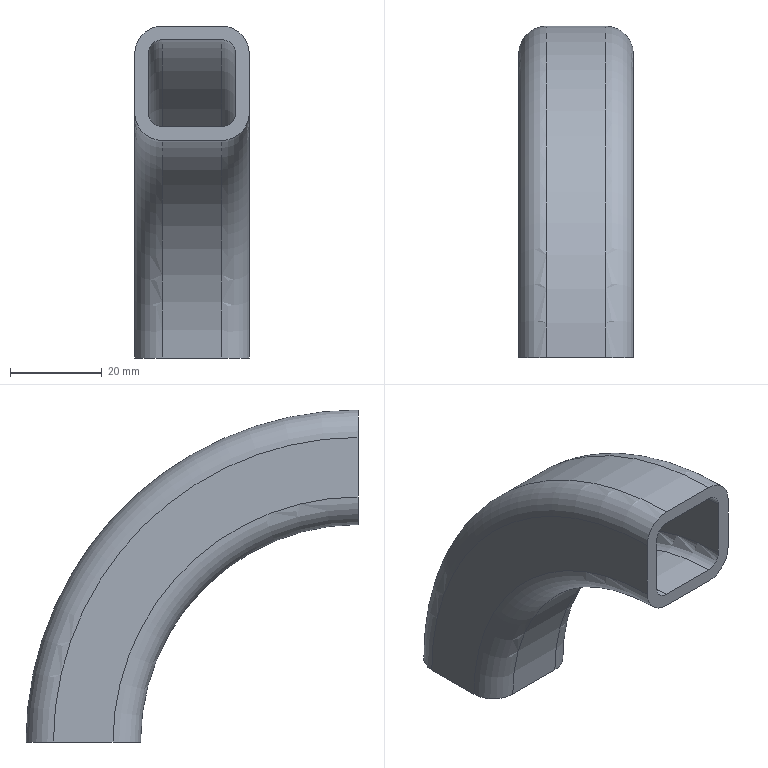Part | STEP file | ISO 10799-2 25x25x3 1784908143949 | 1 solid | 18 faces | box 25 x 72.5 x 72.5 mm | volume 22697 mm3 | torus 8 | plane 6 | cylinder 4 | commonest cylinder face diameters 95 x1 101 x1 139 x1 145 x1
STEP:
#1=CARTESIAN_POINT('',(9.5,-6.5,0.));
#2=VERTEX_POINT('',#1);
#3=CARTESIAN_POINT('',(9.5,6.5,0.));
#4=VERTEX_POINT('',#3);
#5=CARTESIAN_POINT('',(9.5,-3.25,0.));
#6=DIRECTION('',(0.,1.,0.));
#7=VECTOR('',#6,10.);
#8=LINE('',#5,#7);
#9=EDGE_CURVE('',#2,#4,#8,.T.);
#10=ORIENTED_EDGE('',*,*,#9,.F.);
#11=CARTESIAN_POINT('',(9.5,-60.,53.5));
#12=VERTEX_POINT('',#11);
#13=CARTESIAN_POINT('',(9.5,-60.,0.));
#14=DIRECTION('',(1.,0.,0.));
#15=DIRECTION('',(0.,1.,0.));
#16=AXIS2_PLACEMENT_3D('',#13,#14,#15);
#17=CIRCLE('',#16,53.5);
#18=EDGE_CURVE('',#2,#12,#17,.T.);
#19=ORIENTED_EDGE('',*,*,#18,.T.);
#20=CARTESIAN_POINT('',(9.5,-60.,66.5));
#21=VERTEX_POINT('',#20);
#22=CARTESIAN_POINT('',(9.5,-60.,30.));
#23=DIRECTION('',(0.,0.,-1.));
#24=VECTOR('',#23,10.);
#25=LINE('',#22,#24);
#26=EDGE_CURVE('',#21,#12,#25,.T.);
#27=ORIENTED_EDGE('',*,*,#26,.F.);
#28=CARTESIAN_POINT('',(9.5,-60.,0.));
#29=DIRECTION('',(1.,0.,0.));
#30=DIRECTION('',(0.,1.,0.));
#31=AXIS2_PLACEMENT_3D('',#28,#29,#30);
#32=CIRCLE('',#31,66.5);
#33=EDGE_CURVE('',#4,#21,#32,.T.);
#34=ORIENTED_EDGE('',*,*,#33,.F.);
#35=EDGE_LOOP('',(#10,#19,#27,#34));
#36=FACE_OUTER_BOUND('',#35,.T.);
#37=CARTESIAN_POINT('',(9.5,-6.5,0.));
#38=DIRECTION('',(1.,0.,0.));
#39=DIRECTION('',(0.,0.,-1.));
#40=AXIS2_PLACEMENT_3D('',#37,#38,#39);
#41=PLANE('',#40);
#42=ADVANCED_FACE('',(#36),#41,.F.);
#43=CARTESIAN_POINT('',(6.5,-9.5,0.));
#44=VERTEX_POINT('',#43);
#45=CARTESIAN_POINT('',(6.5,-6.5,0.));
#46=DIRECTION('',(0.,0.,1.));
#47=DIRECTION('',(0.,1.,0.));
#48=AXIS2_PLACEMENT_3D('',#45,#46,#47);
#49=CIRCLE('',#48,3.);
#50=EDGE_CURVE('',#44,#2,#49,.T.);
#51=ORIENTED_EDGE('',*,*,#50,.F.);
#52=CARTESIAN_POINT('',(6.5,-60.,50.5));
#53=VERTEX_POINT('',#52);
#54=CARTESIAN_POINT('',(6.5,-60.,0.));
#55=DIRECTION('',(1.,0.,0.));
#56=DIRECTION('',(0.,1.,0.));
#57=AXIS2_PLACEMENT_3D('',#54,#55,#56);
#58=CIRCLE('',#57,50.5);
#59=EDGE_CURVE('',#44,#53,#58,.T.);
#60=ORIENTED_EDGE('',*,*,#59,.T.);
#61=CARTESIAN_POINT('',(6.5,-60.,53.5));
#62=DIRECTION('',(0.,1.,0.));
#63=DIRECTION('',(0.,0.,1.));
#64=AXIS2_PLACEMENT_3D('',#61,#62,#63);
#65=CIRCLE('',#64,3.);
#66=EDGE_CURVE('',#12,#53,#65,.T.);
#67=ORIENTED_EDGE('',*,*,#66,.F.);
#68=ORIENTED_EDGE('',*,*,#18,.F.);
#69=EDGE_LOOP('',(#51,#60,#67,#68));
#70=FACE_OUTER_BOUND('',#69,.T.);
#71=CARTESIAN_POINT('',(6.5,-60.,0.));
#72=DIRECTION('',(1.,0.,0.));
#73=DIRECTION('',(0.,0.,-1.));
#74=AXIS2_PLACEMENT_3D('',#71,#72,#73);
#75=TOROIDAL_SURFACE('',#74,53.5,3.);
#76=ADVANCED_FACE('',(#70),#75,.F.);
#77=CARTESIAN_POINT('',(-6.5,-9.5,0.));
#78=VERTEX_POINT('',#77);
#79=CARTESIAN_POINT('',(0.,-9.5,0.));
#80=DIRECTION('',(1.,0.,0.));
#81=VECTOR('',#80,10.);
#82=LINE('',#79,#81);
#83=EDGE_CURVE('',#78,#44,#82,.T.);
#84=ORIENTED_EDGE('',*,*,#83,.F.);
#85=CARTESIAN_POINT('',(-6.5,-60.,50.5));
#86=VERTEX_POINT('',#85);
#87=CARTESIAN_POINT('',(-6.5,-60.,0.));
#88=DIRECTION('',(1.,0.,0.));
#89=DIRECTION('',(0.,1.,0.));
#90=AXIS2_PLACEMENT_3D('',#87,#88,#89);
#91=CIRCLE('',#90,50.5);
#92=EDGE_CURVE('',#78,#86,#91,.T.);
#93=ORIENTED_EDGE('',*,*,#92,.T.);
#94=CARTESIAN_POINT('',(0.,-60.,50.5));
#95=DIRECTION('',(-1.,0.,0.));
#96=VECTOR('',#95,10.);
#97=LINE('',#94,#96);
#98=EDGE_CURVE('',#53,#86,#97,.T.);
#99=ORIENTED_EDGE('',*,*,#98,.F.);
#100=ORIENTED_EDGE('',*,*,#59,.F.);
#101=EDGE_LOOP('',(#84,#93,#99,#100));
#102=FACE_OUTER_BOUND('',#101,.T.);
#103=CARTESIAN_POINT('',(0.,-60.,0.));
#104=DIRECTION('',(1.,0.,0.));
#105=DIRECTION('',(0.,0.,-1.));
#106=AXIS2_PLACEMENT_3D('',#103,#104,#105);
#107=CYLINDRICAL_SURFACE('',#106,50.5);
#108=ADVANCED_FACE('',(#102),#107,.T.);
#109=CARTESIAN_POINT('',(-9.5,-6.5,0.));
#110=VERTEX_POINT('',#109);
#111=CARTESIAN_POINT('',(-6.5,-6.5,0.));
#112=DIRECTION('',(0.,0.,1.));
#113=DIRECTION('',(0.,1.,0.));
#114=AXIS2_PLACEMENT_3D('',#111,#112,#113);
#115=CIRCLE('',#114,3.);
#116=EDGE_CURVE('',#110,#78,#115,.T.);
#117=ORIENTED_EDGE('',*,*,#116,.F.);
#118=CARTESIAN_POINT('',(-9.5,-60.,53.5));
#119=VERTEX_POINT('',#118);
#120=CARTESIAN_POINT('',(-9.5,-60.,0.));
#121=DIRECTION('',(1.,0.,0.));
#122=DIRECTION('',(0.,1.,0.));
#123=AXIS2_PLACEMENT_3D('',#120,#121,#122);
#124=CIRCLE('',#123,53.5);
#125=EDGE_CURVE('',#110,#119,#124,.T.);
#126=ORIENTED_EDGE('',*,*,#125,.T.);
#127=CARTESIAN_POINT('',(-6.5,-60.,53.5));
#128=DIRECTION('',(0.,1.,0.));
#129=DIRECTION('',(0.,0.,1.));
#130=AXIS2_PLACEMENT_3D('',#127,#128,#129);
#131=CIRCLE('',#130,3.);
#132=EDGE_CURVE('',#86,#119,#131,.T.);
#133=ORIENTED_EDGE('',*,*,#132,.F.);
#134=ORIENTED_EDGE('',*,*,#92,.F.);
#135=EDGE_LOOP('',(#117,#126,#133,#134));
#136=FACE_OUTER_BOUND('',#135,.T.);
#137=CARTESIAN_POINT('',(-6.5,-60.,0.));
#138=DIRECTION('',(1.,0.,0.));
#139=DIRECTION('',(0.,0.,-1.));
#140=AXIS2_PLACEMENT_3D('',#137,#138,#139);
#141=TOROIDAL_SURFACE('',#140,53.5,3.);
#142=ADVANCED_FACE('',(#136),#141,.F.);
#143=CARTESIAN_POINT('',(-9.5,6.5,0.));
#144=VERTEX_POINT('',#143);
#145=CARTESIAN_POINT('',(-9.5,3.25,0.));
#146=DIRECTION('',(0.,-1.,0.));
#147=VECTOR('',#146,10.);
#148=LINE('',#145,#147);
#149=EDGE_CURVE('',#144,#110,#148,.T.);
#150=ORIENTED_EDGE('',*,*,#149,.F.);
#151=CARTESIAN_POINT('',(-9.5,-60.,66.5));
#152=VERTEX_POINT('',#151);
#153=CARTESIAN_POINT('',(-9.5,-60.,0.));
#154=DIRECTION('',(1.,0.,0.));
#155=DIRECTION('',(0.,1.,0.));
#156=AXIS2_PLACEMENT_3D('',#153,#154,#155);
#157=CIRCLE('',#156,66.5);
#158=EDGE_CURVE('',#144,#152,#157,.T.);
#159=ORIENTED_EDGE('',*,*,#158,.T.);
#160=CARTESIAN_POINT('',(-9.5,-60.,30.));
#161=DIRECTION('',(0.,0.,1.));
#162=VECTOR('',#161,10.);
#163=LINE('',#160,#162);
#164=EDGE_CURVE('',#119,#152,#163,.T.);
#165=ORIENTED_EDGE('',*,*,#164,.F.);
#166=ORIENTED_EDGE('',*,*,#125,.F.);
#167=EDGE_LOOP('',(#150,#159,#165,#166));
#168=FACE_OUTER_BOUND('',#167,.T.);
#169=CARTESIAN_POINT('',(-9.5,6.5,0.));
#170=DIRECTION('',(-1.,0.,0.));
#171=DIRECTION('',(0.,0.,1.));
#172=AXIS2_PLACEMENT_3D('',#169,#170,#171);
#173=PLANE('',#172);
#174=ADVANCED_FACE('',(#168),#173,.F.);
#175=CARTESIAN_POINT('',(-6.5,9.5,0.));
#176=VERTEX_POINT('',#175);
#177=CARTESIAN_POINT('',(-6.5,6.5,0.));
#178=DIRECTION('',(0.,0.,1.));
#179=DIRECTION('',(0.,1.,0.));
#180=AXIS2_PLACEMENT_3D('',#177,#178,#179);
#181=CIRCLE('',#180,3.);
#182=EDGE_CURVE('',#176,#144,#181,.T.);
#183=ORIENTED_EDGE('',*,*,#182,.F.);
#184=CARTESIAN_POINT('',(-6.5,-60.,69.5));
#185=VERTEX_POINT('',#184);
#186=CARTESIAN_POINT('',(-6.5,-60.,0.));
#187=DIRECTION('',(1.,0.,0.));
#188=DIRECTION('',(0.,1.,0.));
#189=AXIS2_PLACEMENT_3D('',#186,#187,#188);
#190=CIRCLE('',#189,69.5);
#191=EDGE_CURVE('',#176,#185,#190,.T.);
#192=ORIENTED_EDGE('',*,*,#191,.T.);
#193=CARTESIAN_POINT('',(-6.5,-60.,66.5));
#194=DIRECTION('',(0.,1.,0.));
#195=DIRECTION('',(0.,0.,1.));
#196=AXIS2_PLACEMENT_3D('',#193,#194,#195);
#197=CIRCLE('',#196,3.);
#198=EDGE_CURVE('',#152,#185,#197,.T.);
#199=ORIENTED_EDGE('',*,*,#198,.F.);
#200=ORIENTED_EDGE('',*,*,#158,.F.);
#201=EDGE_LOOP('',(#183,#192,#199,#200));
#202=FACE_OUTER_BOUND('',#201,.T.);
#203=CARTESIAN_POINT('',(-6.5,-60.,0.));
#204=DIRECTION('',(1.,0.,0.));
#205=DIRECTION('',(0.,0.,-1.));
#206=AXIS2_PLACEMENT_3D('',#203,#204,#205);
#207=TOROIDAL_SURFACE('',#206,66.5,3.);
#208=ADVANCED_FACE('',(#202),#207,.F.);
#209=CARTESIAN_POINT('',(6.5,9.5,0.));
#210=VERTEX_POINT('',#209);
#211=CARTESIAN_POINT('',(0.,9.5,0.));
#212=DIRECTION('',(-1.,0.,0.));
#213=VECTOR('',#212,10.);
#214=LINE('',#211,#213);
#215=EDGE_CURVE('',#210,#176,#214,.T.);
#216=ORIENTED_EDGE('',*,*,#215,.F.);
#217=CARTESIAN_POINT('',(6.5,-60.,69.5));
#218=VERTEX_POINT('',#217);
#219=CARTESIAN_POINT('',(6.5,-60.,0.));
#220=DIRECTION('',(1.,0.,0.));
#221=DIRECTION('',(0.,1.,0.));
#222=AXIS2_PLACEMENT_3D('',#219,#220,#221);
#223=CIRCLE('',#222,69.5);
#224=EDGE_CURVE('',#210,#218,#223,.T.);
#225=ORIENTED_EDGE('',*,*,#224,.T.);
#226=CARTESIAN_POINT('',(0.,-60.,69.5));
#227=DIRECTION('',(1.,0.,0.));
#228=VECTOR('',#227,10.);
#229=LINE('',#226,#228);
#230=EDGE_CURVE('',#185,#218,#229,.T.);
#231=ORIENTED_EDGE('',*,*,#230,.F.);
#232=ORIENTED_EDGE('',*,*,#191,.F.);
#233=EDGE_LOOP('',(#216,#225,#231,#232));
#234=FACE_OUTER_BOUND('',#233,.T.);
#235=CARTESIAN_POINT('',(0.,-60.,0.));
#236=DIRECTION('',(1.,0.,0.));
#237=DIRECTION('',(0.,0.,-1.));
#238=AXIS2_PLACEMENT_3D('',#235,#236,#237);
#239=CYLINDRICAL_SURFACE('',#238,69.5);
#240=ADVANCED_FACE('',(#234),#239,.F.);
#241=CARTESIAN_POINT('',(6.5,6.5,0.));
#242=DIRECTION('',(0.,0.,1.));
#243=DIRECTION('',(0.,1.,0.));
#244=AXIS2_PLACEMENT_3D('',#241,#242,#243);
#245=CIRCLE('',#244,3.);
#246=EDGE_CURVE('',#4,#210,#245,.T.);
#247=ORIENTED_EDGE('',*,*,#246,.F.);
#248=ORIENTED_EDGE('',*,*,#33,.T.);
#249=CARTESIAN_POINT('',(6.5,-60.,66.5));
#250=DIRECTION('',(0.,1.,0.));
#251=DIRECTION('',(0.,0.,1.));
#252=AXIS2_PLACEMENT_3D('',#249,#250,#251);
#253=CIRCLE('',#252,3.);
#254=EDGE_CURVE('',#218,#21,#253,.T.);
#255=ORIENTED_EDGE('',*,*,#254,.F.);
#256=ORIENTED_EDGE('',*,*,#224,.F.);
#257=EDGE_LOOP('',(#247,#248,#255,#256));
#258=FACE_OUTER_BOUND('',#257,.T.);
#259=CARTESIAN_POINT('',(6.5,-60.,0.));
#260=DIRECTION('',(1.,0.,0.));
#261=DIRECTION('',(0.,0.,-1.));
#262=AXIS2_PLACEMENT_3D('',#259,#260,#261);
#263=TOROIDAL_SURFACE('',#262,66.5,3.);
#264=ADVANCED_FACE('',(#258),#263,.F.);
#265=CARTESIAN_POINT('',(-6.5,-12.5,0.));
#266=VERTEX_POINT('',#265);
#267=CARTESIAN_POINT('',(6.5,-12.5,0.));
#268=VERTEX_POINT('',#267);
#269=CARTESIAN_POINT('',(-6.5,-12.5,0.));
#270=DIRECTION('',(1.,0.,0.));
#271=VECTOR('',#270,10.);
#272=LINE('',#269,#271);
#273=EDGE_CURVE('',#266,#268,#272,.T.);
#274=ORIENTED_EDGE('',*,*,#273,.T.);
#275=CARTESIAN_POINT('',(6.5,-60.,47.5));
#276=VERTEX_POINT('',#275);
#277=CARTESIAN_POINT('',(6.5,-60.,0.));
#278=DIRECTION('',(1.,0.,0.));
#279=DIRECTION('',(0.,1.,0.));
#280=AXIS2_PLACEMENT_3D('',#277,#278,#279);
#281=CIRCLE('',#280,47.5);
#282=EDGE_CURVE('',#268,#276,#281,.T.);
#283=ORIENTED_EDGE('',*,*,#282,.T.);
#284=CARTESIAN_POINT('',(-6.5,-60.,47.5));
#285=VERTEX_POINT('',#284);
#286=CARTESIAN_POINT('',(-6.5,-60.,47.5));
#287=DIRECTION('',(1.,0.,0.));
#288=VECTOR('',#287,10.);
#289=LINE('',#286,#288);
#290=EDGE_CURVE('',#285,#276,#289,.T.);
#291=ORIENTED_EDGE('',*,*,#290,.F.);
#292=CARTESIAN_POINT('',(-6.5,-60.,0.));
#293=DIRECTION('',(1.,0.,0.));
#294=DIRECTION('',(0.,1.,0.));
#295=AXIS2_PLACEMENT_3D('',#292,#293,#294);
#296=CIRCLE('',#295,47.5);
#297=EDGE_CURVE('',#266,#285,#296,.T.);
#298=ORIENTED_EDGE('',*,*,#297,.F.);
#299=EDGE_LOOP('',(#274,#283,#291,#298));
#300=FACE_OUTER_BOUND('',#299,.T.);
#301=CARTESIAN_POINT('',(0.,-60.,0.));
#302=DIRECTION('',(1.,0.,0.));
#303=DIRECTION('',(0.,0.,-1.));
#304=AXIS2_PLACEMENT_3D('',#301,#302,#303);
#305=CYLINDRICAL_SURFACE('',#304,47.5);
#306=ADVANCED_FACE('',(#300),#305,.F.);
#307=CARTESIAN_POINT('',(-12.5,-6.5,0.));
#308=VERTEX_POINT('',#307);
#309=CARTESIAN_POINT('',(-6.5,-6.5,0.));
#310=DIRECTION('',(0.,0.,1.));
#311=DIRECTION('',(0.,1.,0.));
#312=AXIS2_PLACEMENT_3D('',#309,#310,#311);
#313=CIRCLE('',#312,6.);
#314=EDGE_CURVE('',#308,#266,#313,.T.);
#315=ORIENTED_EDGE('',*,*,#314,.T.);
#316=ORIENTED_EDGE('',*,*,#297,.T.);
#317=CARTESIAN_POINT('',(-12.5,-60.,53.5));
#318=VERTEX_POINT('',#317);
#319=CARTESIAN_POINT('',(-6.5,-60.,53.5));
#320=DIRECTION('',(0.,-1.,0.));
#321=DIRECTION('',(0.,0.,1.));
#322=AXIS2_PLACEMENT_3D('',#319,#320,#321);
#323=CIRCLE('',#322,6.);
#324=EDGE_CURVE('',#318,#285,#323,.T.);
#325=ORIENTED_EDGE('',*,*,#324,.F.);
#326=CARTESIAN_POINT('',(-12.5,-60.,0.));
#327=DIRECTION('',(1.,0.,0.));
#328=DIRECTION('',(0.,1.,0.));
#329=AXIS2_PLACEMENT_3D('',#326,#327,#328);
#330=CIRCLE('',#329,53.5);
#331=EDGE_CURVE('',#308,#318,#330,.T.);
#332=ORIENTED_EDGE('',*,*,#331,.F.);
#333=EDGE_LOOP('',(#315,#316,#325,#332));
#334=FACE_OUTER_BOUND('',#333,.T.);
#335=CARTESIAN_POINT('',(-6.5,-60.,0.));
#336=DIRECTION('',(1.,0.,0.));
#337=DIRECTION('',(0.,0.,-1.));
#338=AXIS2_PLACEMENT_3D('',#335,#336,#337);
#339=TOROIDAL_SURFACE('',#338,53.5,6.);
#340=ADVANCED_FACE('',(#334),#339,.T.);
#341=CARTESIAN_POINT('',(-12.5,6.5,0.));
#342=VERTEX_POINT('',#341);
#343=CARTESIAN_POINT('',(-12.5,6.5,0.));
#344=DIRECTION('',(0.,-1.,0.));
#345=VECTOR('',#344,10.);
#346=LINE('',#343,#345);
#347=EDGE_CURVE('',#342,#308,#346,.T.);
#348=ORIENTED_EDGE('',*,*,#347,.T.);
#349=ORIENTED_EDGE('',*,*,#331,.T.);
#350=CARTESIAN_POINT('',(-12.5,-60.,66.5));
#351=VERTEX_POINT('',#350);
#352=CARTESIAN_POINT('',(-12.5,-60.,66.5));
#353=DIRECTION('',(0.,0.,-1.));
#354=VECTOR('',#353,10.);
#355=LINE('',#352,#354);
#356=EDGE_CURVE('',#351,#318,#355,.T.);
#357=ORIENTED_EDGE('',*,*,#356,.F.);
#358=CARTESIAN_POINT('',(-12.5,-60.,0.));
#359=DIRECTION('',(1.,0.,0.));
#360=DIRECTION('',(0.,1.,0.));
#361=AXIS2_PLACEMENT_3D('',#358,#359,#360);
#362=CIRCLE('',#361,66.5);
#363=EDGE_CURVE('',#342,#351,#362,.T.);
#364=ORIENTED_EDGE('',*,*,#363,.F.);
#365=EDGE_LOOP('',(#348,#349,#357,#364));
#366=FACE_OUTER_BOUND('',#365,.T.);
#367=CARTESIAN_POINT('',(-12.5,6.5,0.));
#368=DIRECTION('',(-1.,0.,0.));
#369=DIRECTION('',(0.,0.,1.));
#370=AXIS2_PLACEMENT_3D('',#367,#368,#369);
#371=PLANE('',#370);
#372=ADVANCED_FACE('',(#366),#371,.T.);
#373=CARTESIAN_POINT('',(-6.5,12.5,0.));
#374=VERTEX_POINT('',#373);
#375=CARTESIAN_POINT('',(-6.5,6.5,0.));
#376=DIRECTION('',(0.,0.,1.));
#377=DIRECTION('',(1.,0.,0.));
#378=AXIS2_PLACEMENT_3D('',#375,#376,#377);
#379=CIRCLE('',#378,6.);
#380=EDGE_CURVE('',#374,#342,#379,.T.);
#381=ORIENTED_EDGE('',*,*,#380,.T.);
#382=ORIENTED_EDGE('',*,*,#363,.T.);
#383=CARTESIAN_POINT('',(-6.5,-60.,72.5));
#384=VERTEX_POINT('',#383);
#385=CARTESIAN_POINT('',(-6.5,-60.,66.5));
#386=DIRECTION('',(0.,-1.,0.));
#387=DIRECTION('',(1.,0.,0.));
#388=AXIS2_PLACEMENT_3D('',#385,#386,#387);
#389=CIRCLE('',#388,6.);
#390=EDGE_CURVE('',#384,#351,#389,.T.);
#391=ORIENTED_EDGE('',*,*,#390,.F.);
#392=CARTESIAN_POINT('',(-6.5,-60.,0.));
#393=DIRECTION('',(1.,0.,0.));
#394=DIRECTION('',(0.,1.,0.));
#395=AXIS2_PLACEMENT_3D('',#392,#393,#394);
#396=CIRCLE('',#395,72.5);
#397=EDGE_CURVE('',#374,#384,#396,.T.);
#398=ORIENTED_EDGE('',*,*,#397,.F.);
#399=EDGE_LOOP('',(#381,#382,#391,#398));
#400=FACE_OUTER_BOUND('',#399,.T.);
#401=CARTESIAN_POINT('',(-6.5,-60.,0.));
#402=DIRECTION('',(1.,0.,0.));
#403=DIRECTION('',(0.,0.,-1.));
#404=AXIS2_PLACEMENT_3D('',#401,#402,#403);
#405=TOROIDAL_SURFACE('',#404,66.5,6.);
#406=ADVANCED_FACE('',(#400),#405,.T.);
#407=CARTESIAN_POINT('',(6.5,12.5,0.));
#408=VERTEX_POINT('',#407);
#409=CARTESIAN_POINT('',(6.5,12.5,0.));
#410=DIRECTION('',(-1.,0.,0.));
#411=VECTOR('',#410,10.);
#412=LINE('',#409,#411);
#413=EDGE_CURVE('',#408,#374,#412,.T.);
#414=ORIENTED_EDGE('',*,*,#413,.T.);
#415=ORIENTED_EDGE('',*,*,#397,.T.);
#416=CARTESIAN_POINT('',(6.5,-60.,72.5));
#417=VERTEX_POINT('',#416);
#418=CARTESIAN_POINT('',(6.5,-60.,72.5));
#419=DIRECTION('',(-1.,0.,0.));
#420=VECTOR('',#419,10.);
#421=LINE('',#418,#420);
#422=EDGE_CURVE('',#417,#384,#421,.T.);
#423=ORIENTED_EDGE('',*,*,#422,.F.);
#424=CARTESIAN_POINT('',(6.5,-60.,0.));
#425=DIRECTION('',(1.,0.,0.));
#426=DIRECTION('',(0.,1.,0.));
#427=AXIS2_PLACEMENT_3D('',#424,#425,#426);
#428=CIRCLE('',#427,72.5);
#429=EDGE_CURVE('',#408,#417,#428,.T.);
#430=ORIENTED_EDGE('',*,*,#429,.F.);
#431=EDGE_LOOP('',(#414,#415,#423,#430));
#432=FACE_OUTER_BOUND('',#431,.T.);
#433=CARTESIAN_POINT('',(0.,-60.,0.));
#434=DIRECTION('',(1.,0.,0.));
#435=DIRECTION('',(0.,0.,-1.));
#436=AXIS2_PLACEMENT_3D('',#433,#434,#435);
#437=CYLINDRICAL_SURFACE('',#436,72.5);
#438=ADVANCED_FACE('',(#432),#437,.T.);
#439=CARTESIAN_POINT('',(12.5,6.5,0.));
#440=VERTEX_POINT('',#439);
#441=CARTESIAN_POINT('',(6.5,6.5,0.));
#442=DIRECTION('',(0.,0.,1.));
#443=DIRECTION('',(0.,-1.,0.));
#444=AXIS2_PLACEMENT_3D('',#441,#442,#443);
#445=CIRCLE('',#444,6.);
#446=EDGE_CURVE('',#440,#408,#445,.T.);
#447=ORIENTED_EDGE('',*,*,#446,.T.);
#448=ORIENTED_EDGE('',*,*,#429,.T.);
#449=CARTESIAN_POINT('',(12.5,-60.,66.5));
#450=VERTEX_POINT('',#449);
#451=CARTESIAN_POINT('',(6.5,-60.,66.5));
#452=DIRECTION('',(0.,-1.,0.));
#453=DIRECTION('',(0.,0.,-1.));
#454=AXIS2_PLACEMENT_3D('',#451,#452,#453);
#455=CIRCLE('',#454,6.);
#456=EDGE_CURVE('',#450,#417,#455,.T.);
#457=ORIENTED_EDGE('',*,*,#456,.F.);
#458=CARTESIAN_POINT('',(12.5,-60.,0.));
#459=DIRECTION('',(1.,0.,0.));
#460=DIRECTION('',(0.,1.,0.));
#461=AXIS2_PLACEMENT_3D('',#458,#459,#460);
#462=CIRCLE('',#461,66.5);
#463=EDGE_CURVE('',#440,#450,#462,.T.);
#464=ORIENTED_EDGE('',*,*,#463,.F.);
#465=EDGE_LOOP('',(#447,#448,#457,#464));
#466=FACE_OUTER_BOUND('',#465,.T.);
#467=CARTESIAN_POINT('',(6.5,-60.,0.));
#468=DIRECTION('',(1.,0.,0.));
#469=DIRECTION('',(0.,0.,-1.));
#470=AXIS2_PLACEMENT_3D('',#467,#468,#469);
#471=TOROIDAL_SURFACE('',#470,66.5,6.);
#472=ADVANCED_FACE('',(#466),#471,.T.);
#473=CARTESIAN_POINT('',(12.5,-6.5,0.));
#474=VERTEX_POINT('',#473);
#475=CARTESIAN_POINT('',(12.5,-6.5,0.));
#476=DIRECTION('',(0.,1.,0.));
#477=VECTOR('',#476,10.);
#478=LINE('',#475,#477);
#479=EDGE_CURVE('',#474,#440,#478,.T.);
#480=ORIENTED_EDGE('',*,*,#479,.T.);
#481=ORIENTED_EDGE('',*,*,#463,.T.);
#482=CARTESIAN_POINT('',(12.5,-60.,53.5));
#483=VERTEX_POINT('',#482);
#484=CARTESIAN_POINT('',(12.5,-60.,53.5));
#485=DIRECTION('',(0.,0.,1.));
#486=VECTOR('',#485,10.);
#487=LINE('',#484,#486);
#488=EDGE_CURVE('',#483,#450,#487,.T.);
#489=ORIENTED_EDGE('',*,*,#488,.F.);
#490=CARTESIAN_POINT('',(12.5,-60.,0.));
#491=DIRECTION('',(1.,0.,0.));
#492=DIRECTION('',(0.,1.,0.));
#493=AXIS2_PLACEMENT_3D('',#490,#491,#492);
#494=CIRCLE('',#493,53.5);
#495=EDGE_CURVE('',#474,#483,#494,.T.);
#496=ORIENTED_EDGE('',*,*,#495,.F.);
#497=EDGE_LOOP('',(#480,#481,#489,#496));
#498=FACE_OUTER_BOUND('',#497,.T.);
#499=CARTESIAN_POINT('',(12.5,-6.5,0.));
#500=DIRECTION('',(1.,0.,0.));
#501=DIRECTION('',(0.,0.,-1.));
#502=AXIS2_PLACEMENT_3D('',#499,#500,#501);
#503=PLANE('',#502);
#504=ADVANCED_FACE('',(#498),#503,.T.);
#505=CARTESIAN_POINT('',(6.5,-6.5,0.));
#506=DIRECTION('',(0.,0.,1.));
#507=DIRECTION('',(-1.,0.,0.));
#508=AXIS2_PLACEMENT_3D('',#505,#506,#507);
#509=CIRCLE('',#508,6.);
#510=EDGE_CURVE('',#268,#474,#509,.T.);
#511=ORIENTED_EDGE('',*,*,#510,.T.);
#512=ORIENTED_EDGE('',*,*,#495,.T.);
#513=CARTESIAN_POINT('',(6.5,-60.,53.5));
#514=DIRECTION('',(0.,-1.,0.));
#515=DIRECTION('',(-1.,0.,0.));
#516=AXIS2_PLACEMENT_3D('',#513,#514,#515);
#517=CIRCLE('',#516,6.);
#518=EDGE_CURVE('',#276,#483,#517,.T.);
#519=ORIENTED_EDGE('',*,*,#518,.F.);
#520=ORIENTED_EDGE('',*,*,#282,.F.);
#521=EDGE_LOOP('',(#511,#512,#519,#520));
#522=FACE_OUTER_BOUND('',#521,.T.);
#523=CARTESIAN_POINT('',(6.5,-60.,0.));
#524=DIRECTION('',(1.,0.,0.));
#525=DIRECTION('',(0.,0.,-1.));
#526=AXIS2_PLACEMENT_3D('',#523,#524,#525);
#527=TOROIDAL_SURFACE('',#526,53.5,6.);
#528=ADVANCED_FACE('',(#522),#527,.T.);
#529=ORIENTED_EDGE('',*,*,#518,.T.);
#530=ORIENTED_EDGE('',*,*,#488,.T.);
#531=ORIENTED_EDGE('',*,*,#456,.T.);
#532=ORIENTED_EDGE('',*,*,#422,.T.);
#533=ORIENTED_EDGE('',*,*,#390,.T.);
#534=ORIENTED_EDGE('',*,*,#356,.T.);
#535=ORIENTED_EDGE('',*,*,#324,.T.);
#536=ORIENTED_EDGE('',*,*,#290,.T.);
#537=EDGE_LOOP('',(#529,#530,#531,#532,#533,#534,#535,#536));
#538=FACE_OUTER_BOUND('',#537,.T.);
#539=ORIENTED_EDGE('',*,*,#26,.T.);
#540=ORIENTED_EDGE('',*,*,#66,.T.);
#541=ORIENTED_EDGE('',*,*,#98,.T.);
#542=ORIENTED_EDGE('',*,*,#132,.T.);
#543=ORIENTED_EDGE('',*,*,#164,.T.);
#544=ORIENTED_EDGE('',*,*,#198,.T.);
#545=ORIENTED_EDGE('',*,*,#230,.T.);
#546=ORIENTED_EDGE('',*,*,#254,.T.);
#547=EDGE_LOOP('',(#539,#540,#541,#542,#543,#544,#545,#546));
#548=FACE_BOUND('',#547,.T.);
#549=CARTESIAN_POINT('',(0.,-60.,60.));
#550=DIRECTION('',(0.,-1.,0.));
#551=DIRECTION('',(1.,0.,0.));
#552=AXIS2_PLACEMENT_3D('',#549,#550,#551);
#553=PLANE('',#552);
#554=ADVANCED_FACE('',(#538,#548),#553,.T.);
#555=ORIENTED_EDGE('',*,*,#510,.F.);
#556=ORIENTED_EDGE('',*,*,#273,.F.);
#557=ORIENTED_EDGE('',*,*,#314,.F.);
#558=ORIENTED_EDGE('',*,*,#347,.F.);
#559=ORIENTED_EDGE('',*,*,#380,.F.);
#560=ORIENTED_EDGE('',*,*,#413,.F.);
#561=ORIENTED_EDGE('',*,*,#446,.F.);
#562=ORIENTED_EDGE('',*,*,#479,.F.);
#563=EDGE_LOOP('',(#555,#556,#557,#558,#559,#560,#561,#562));
#564=FACE_OUTER_BOUND('',#563,.T.);
#565=ORIENTED_EDGE('',*,*,#9,.T.);
#566=ORIENTED_EDGE('',*,*,#246,.T.);
#567=ORIENTED_EDGE('',*,*,#215,.T.);
#568=ORIENTED_EDGE('',*,*,#182,.T.);
#569=ORIENTED_EDGE('',*,*,#149,.T.);
#570=ORIENTED_EDGE('',*,*,#116,.T.);
#571=ORIENTED_EDGE('',*,*,#83,.T.);
#572=ORIENTED_EDGE('',*,*,#50,.T.);
#573=EDGE_LOOP('',(#565,#566,#567,#568,#569,#570,#571,#572));
#574=FACE_BOUND('',#573,.T.);
#575=CARTESIAN_POINT('',(0.,0.,0.));
#576=DIRECTION('',(0.,0.,1.));
#577=DIRECTION('',(1.,0.,0.));
#578=AXIS2_PLACEMENT_3D('',#575,#576,#577);
#579=PLANE('',#578);
#580=ADVANCED_FACE('',(#564,#574),#579,.F.);
#581=CLOSED_SHELL('',(#42,#76,#108,#142,#174,#208,#240,#264,#306,#340,#372,#406,#438,#472,#504,#528,#554,#580));
#582=MANIFOLD_SOLID_BREP('',#581);
#583=(LENGTH_UNIT()NAMED_UNIT(*)SI_UNIT(.MILLI.,.METRE.));
#584=UNCERTAINTY_MEASURE_WITH_UNIT(LENGTH_MEASURE(0.01),#583,'','');
#585=(NAMED_UNIT(*)PLANE_ANGLE_UNIT()SI_UNIT($,.RADIAN.));
#586=(NAMED_UNIT(*)SI_UNIT($,.STERADIAN.)SOLID_ANGLE_UNIT());
#587=(GEOMETRIC_REPRESENTATION_CONTEXT(3)GLOBAL_UNCERTAINTY_ASSIGNED_CONTEXT((#584))GLOBAL_UNIT_ASSIGNED_CONTEXT((#583,#585,#586))REPRESENTATION_CONTEXT('',''));
#588=ADVANCED_BREP_SHAPE_REPRESENTATION('',(#582),#587);